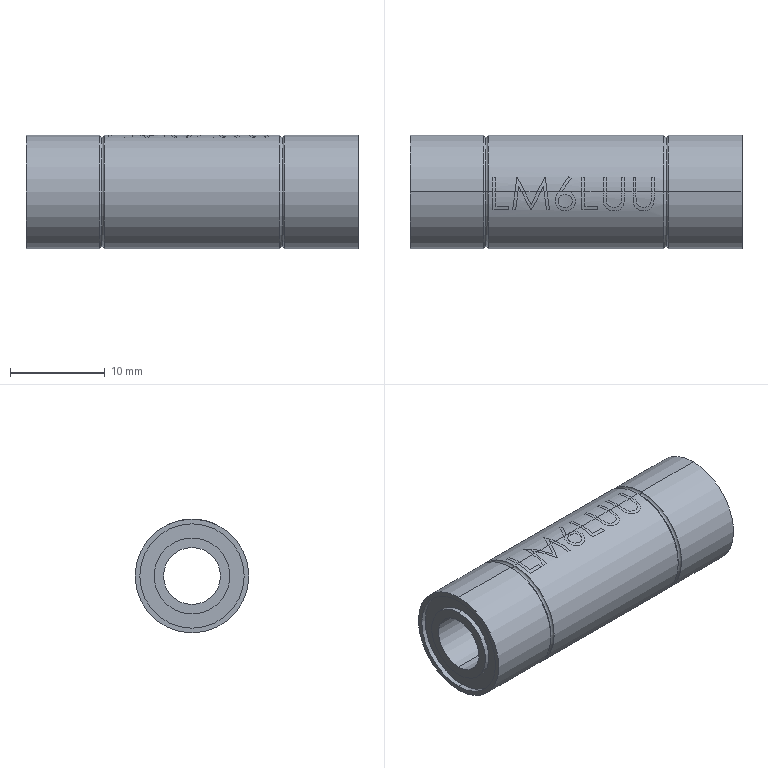Part | SolidWorks | features Emboss 1, Revolution 1 | 1 solid | 53 faces | box 35 x 12 x 12 mm | volume 2917 mm3 | cylinder 39 | torus 8 | plane 6 | commonest cylinder face diameters 12 x29 8 x4 11 x4 6 x2